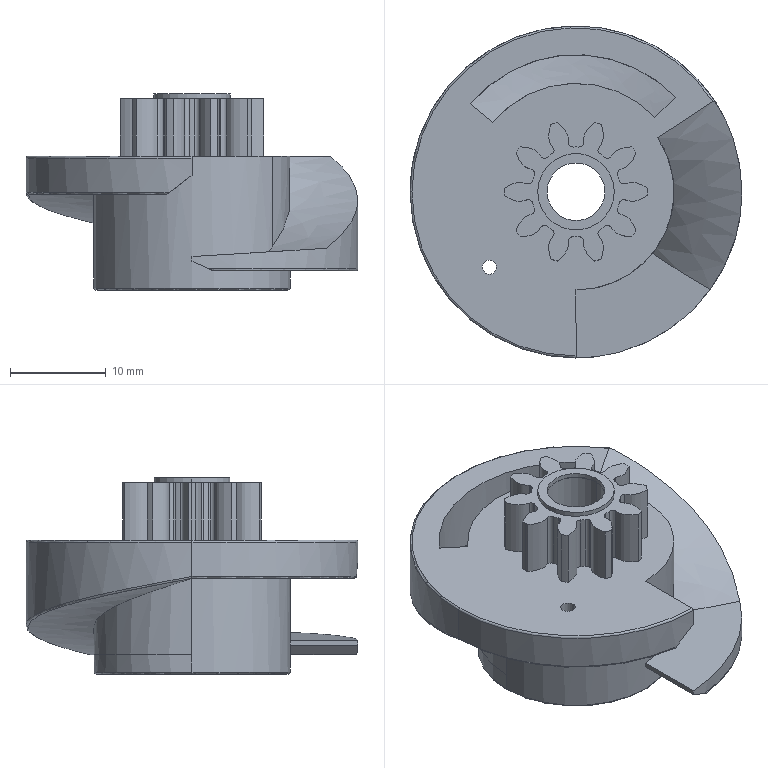Part | SolidWorks | features ICE 12, Chamfer 4, Fillet 4, CirPattern 2, Helix 2, SweepCut 2, Extrusion 1, RefAxis 1 | 1 solid | 136 faces | box 34.7 x 34.7 x 20.5 mm | volume 6291 mm3 | cylinder 70 | plane 28 | spline 28 | torus 7 | cone 2 | sphere 1 | commonest cylinder face diameters 0.95 x24 15 x11 9.375 x10 11 x4 16.4 x4 34.7 x3